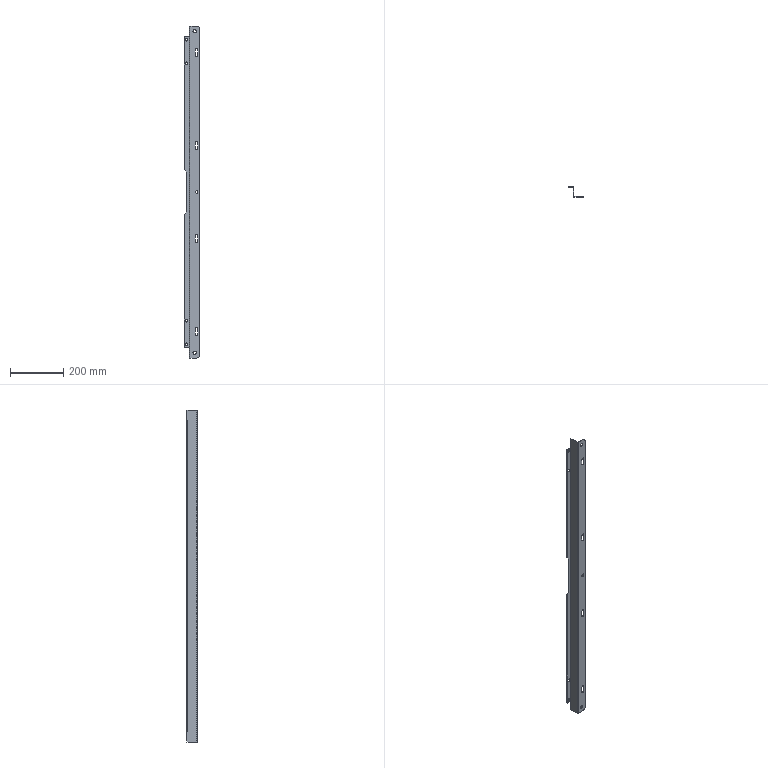Part | SolidWorks | features ICE 3, Cut 2, SMBaseFlange 2, Chamfer 1, Fillet 1, FlatPattern 1, SheetMetal 1 | 1 solid | 70 faces | box 60 x 38 x 1250 mm | volume 171739 mm3 | plane 38 | cylinder 32 | commonest cylinder face diameters 10 x14 11 x8 12.8 x4 0.4 x2 3.4 x2 26 x2